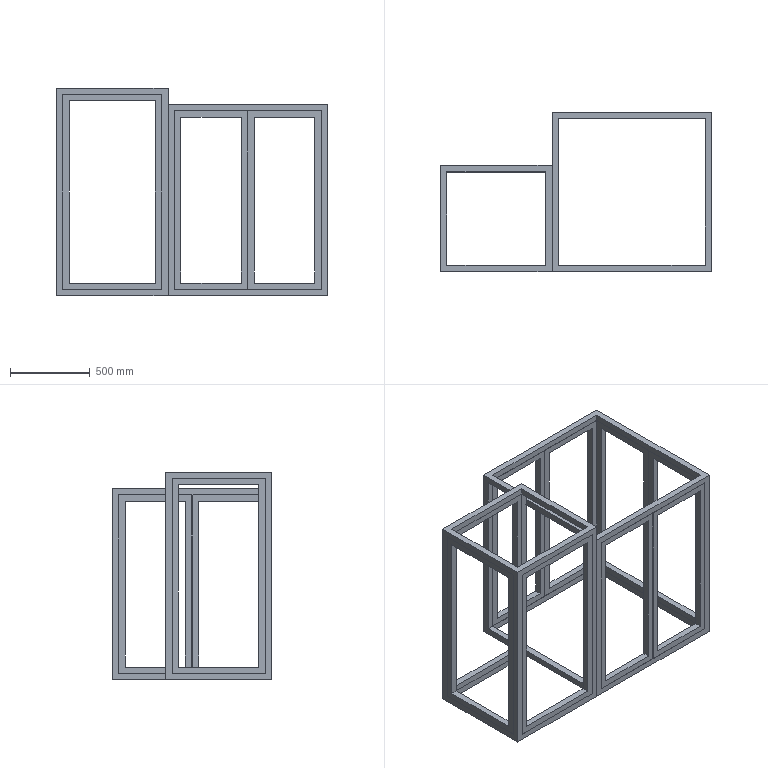Part | STEP file | Upper frame | 11 solids | 146 faces | box 1700 x 1000 x 1302 mm | volume 80127840 mm3 | plane 146